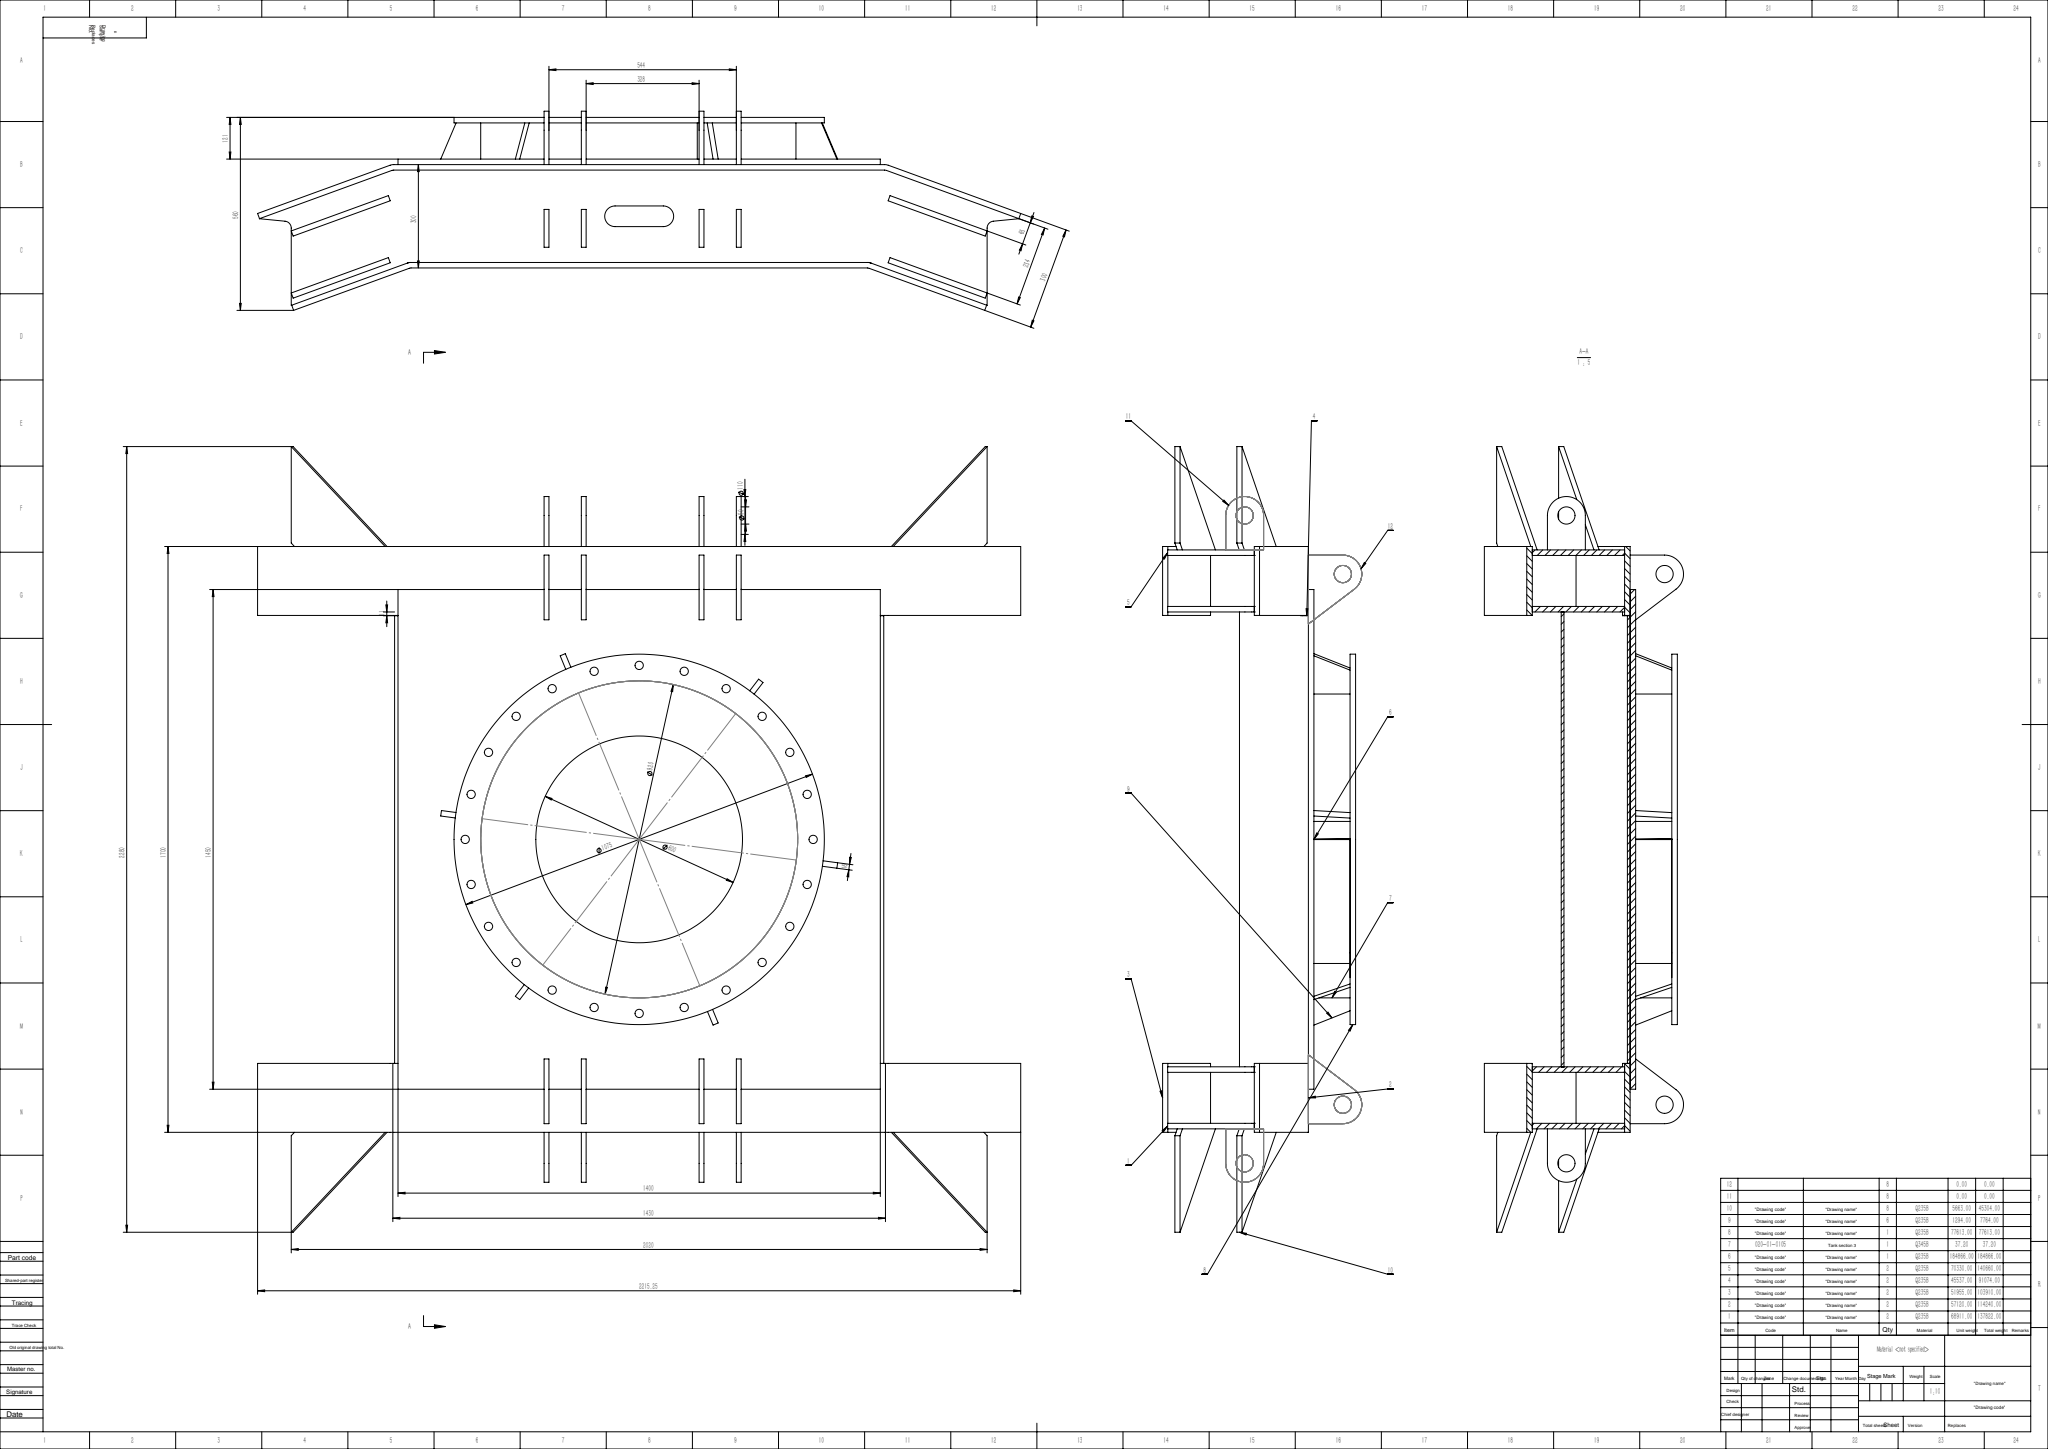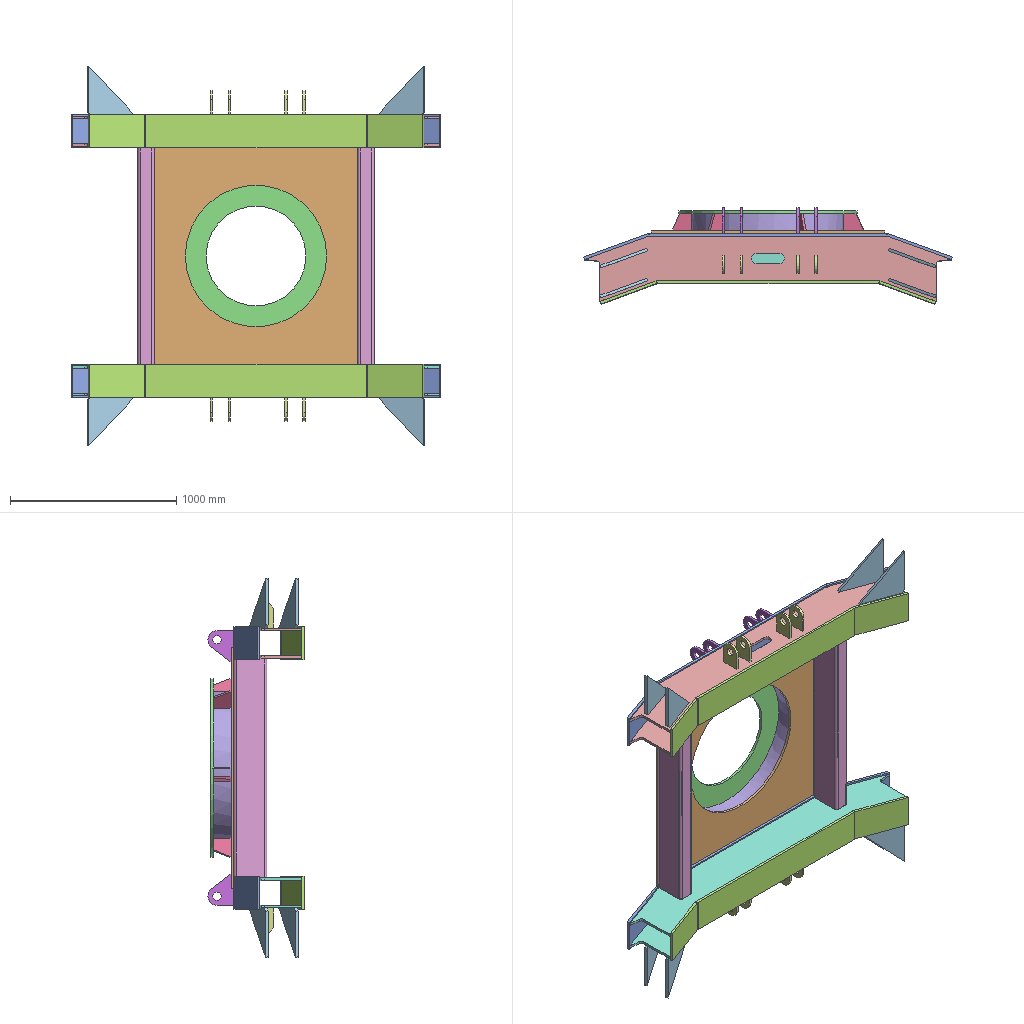Assembly | SolidWorks | 12 different items | 43 placed | box 2215 x 578 x 2280 mm
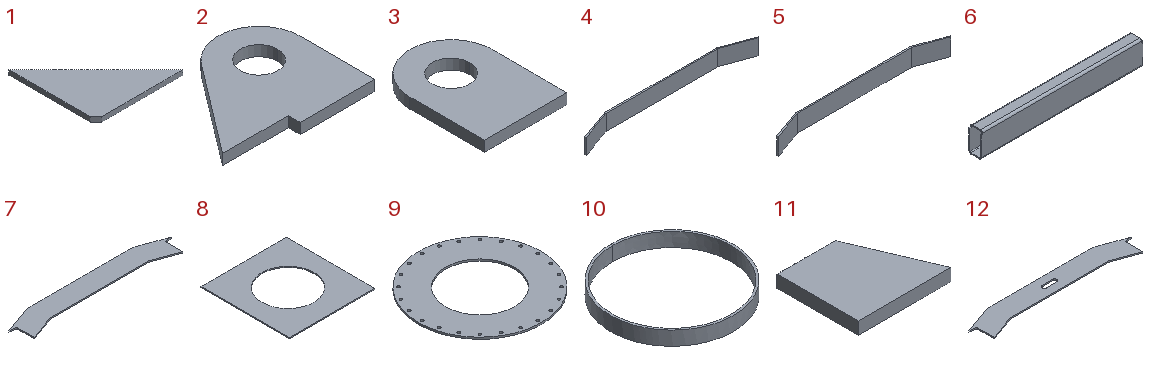Parts list (item | quantity | size | volume | features):
1 | x8 | 300 x 300 x 16 mm | 716800 mm3 | features Chamfer 1, Extrusion 1
2 | x8 | 187.85 x 155 x 14 mm | 247165 mm3 | features Extrusion 1, ICE 1
3 | x8 | 110 x 155 x 14 mm | 193034 mm3 | features Extrusion 1
4 | x2 | 2215 x 156.912 x 200 mm | 7230328 mm3 | features FlatPattern 1, SMBaseFlange 1, SheetMetal 1
5 | x2 | 2017 x 139.101 x 200 mm | 6576544 mm3 | features FlatPattern 1, SMBaseFlange 1, SheetMetal 1
6 | x2 | 1321 x 100 x 200 mm | 5764189 mm3 | features ICE 1, MirrorPattern 1, WeldMemberFeat 1, WeldmentFeature 1
7 | x2 | 2205 x 392.571 x 16 mm | 8902489 mm3 | features Fillet 1, FlatPattern 1, ICE 1, SMBaseFlange 1, SheetMetal 1
8 | x1 | 1400 x 1450 x 16 mm | 23400797 mm3 | features FlatPattern 1, ICE 1, SMBaseFlange 1, SheetMetal 1
9 | x1 | 1075 x 1075 x 16 mm | 9824401 mm3 | features CirPattern 1, FlatPattern 1, HoleWzd 1, ICE 1, SMBaseFlange 1, SheetMetal 1
10 | x1 | 920 x 920.001 x 105 mm | 4770127 mm3 | features FlatPattern 1, LoftedBend 1, SheetMetal 1
11 | x6 | 120 x 105 x 16 mm | 163800 mm3 | features Extrusion 1
12 | x2 | 2205 x 392.571 x 16 mm | 8722850 mm3 | features ICE 2, Fillet 1, FlatPattern 1, SMBaseFlange 1, SheetMetal 1
Mates (type | each side: item.copy, entity, surface, feature):
Coincident | 12.1 face plane Base-Flange1 | 12.2 face plane Base-Flange1
Coincident | 12.1 plane | 12.2 plane
DistanceDim | 12.2 face plane Base-Flange1 | 12.1 face plane Base-Flange1
Coincident | 12.2 face plane Base-Flange1 | 4.1 face plane Base-Flange1
Coincident | 12.1 plane | 4.1 plane
Width | 4.1 face plane Base-Flange1 | 4.1 face plane Base-Flange1 | 12.2 face plane Base-Flange1 | 12.1 face plane Base-Flange1
Coincident | 12.2 face plane Base-Flange1 | 5.1 face plane Base-Flange1
Width | 5.1 face plane Base-Flange1 | 5.1 face plane Base-Flange1 | 12.1 face plane Base-Flange1 | 12.2 face plane Base-Flange1
Coincident | 12.1 plane | 5.1 plane
Coincident | 12.1 face plane Base-Flange1 | 7.1 face plane Base-Flange1
Coincident | 12.1 plane | 7.1 plane
Coincident | 7.1 face plane Base-Flange1 | 7.2 face plane Base-Flange1
DistanceDim | 7.2 face plane Base-Flange1 | 7.1 face plane Base-Flange1
Coincident | 12.1 plane | 7.2 plane
DistanceDim | 7.2 face plane Base-Flange1 | 12.1 face plane Base-Flange1
Coincident | 7.1 face plane Base-Flange1 | 4.2 face plane Base-Flange1
Width | 4.2 face plane Base-Flange1 | 4.2 face plane Base-Flange1 | 7.2 face plane Base-Flange1 | 7.1 face plane Base-Flange1
Coincident | 12.1 plane | 4.2 plane
Coincident | 7.1 face plane Base-Flange1 | 5.2 face plane Base-Flange1
Width | 5.2 face plane Base-Flange1 | 5.2 face plane Base-Flange1 | 7.1 face plane Base-Flange1 | 7.2 face plane Base-Flange1
Coincident | 12.1 plane | 5.2 plane
Coincident | 6.1 face plane Structural cold-formed rectangular hollow section (gb t6728-2002) 200×100×8(1) | 4.2 face plane Base-Flange1
Coincident | 6.1 face plane Structural cold-formed rectangular hollow section (gb t6728-2002) 200×100×8(1) | 7.1 face plane Base-Flange1
Coincident | 6.2 face plane Structural cold-formed rectangular hollow section (gb t6728-2002) 200×100×8(1) | 8.1 face plane Base-Flange1
Width | 8.1 face plane Base-Flange1 | 8.1 face plane Base-Flange1 | 4.2 face plane Base-Flange1 | 4.1 face plane Base-Flange1
Concentric | assembly face | assembly face
Coincident | assembly face | assembly face
Coincident | 12.1 plane | assembly plane
Symmetric | 8.1 face plane Base-Flange1 | 8.1 face plane Base-Flange1 | assembly plane
DistanceDim | assembly plane | 6.1 face plane Structural cold-formed rectangular hollow section (gb t6728-2002) 200×100×8(1)
Coincident | 8.1 plane | assembly plane
Concentric | 8.1 face cylinder Cut-Extrude1 | 10.1 select_type:24
Parallel | 8.1 face plane Base-Flange1 | 10.1 plane
Tangent | 8.1 face plane Base-Flange1 | 10.1 face surface:4006 Freeform bend1
Concentric | 8.1 face cylinder Cut-Extrude1 | 9.1 face cylinder Cut-Extrude1
Tangent | 10.1 face surface:4006 Freeform bend1 | 9.1 face plane Base-Flange1
Concentric | 9.1 face cylinder Cut-Extrude1 | 11.1 select_type:24
Coincident | 9.1 face plane Base-Flange1 | 11.1 face plane Boss-Extrude1
PlanarAngleDim | 9.1 plane | 11.1 plane
Parallel | 8.1 face plane Base-Flange1 | 9.1 plane
Coincident | 7.2 face plane Base-Flange1 | 1.1 face plane Boss-Extrude1
DistanceDim | 1.1 face plane Boss-Extrude1 | 4.2 face plane Base-Flange1
Coincident | 7.2 face plane Cut-Extrude1 | 1.1 edge
Coincident | 7.2 face plane Base-Flange1 | 3.1 face plane Boss-Extrude1
DistanceDim | 3.1 face plane Boss-Extrude1 | 5.2 face plane Base-Flange1
DistanceDim | 3.1 face plane Boss-Extrude1 | 6.2 face plane Structural cold-formed rectangular hollow section (gb t6728-2002) 200×100×8(1)
Coincident | 4.2 face plane Base-Flange1 | 2.1 face plane Boss-Extrude1
Width | 2.2 face plane Boss-Extrude1 | 2.1 face plane Boss-Extrude1 | 3.1 face plane Boss-Extrude1 | 3.2 face plane Boss-Extrude1
DistanceDim | 2.1 face plane Boss-Extrude1 | 4.2 face plane Base-Flange1